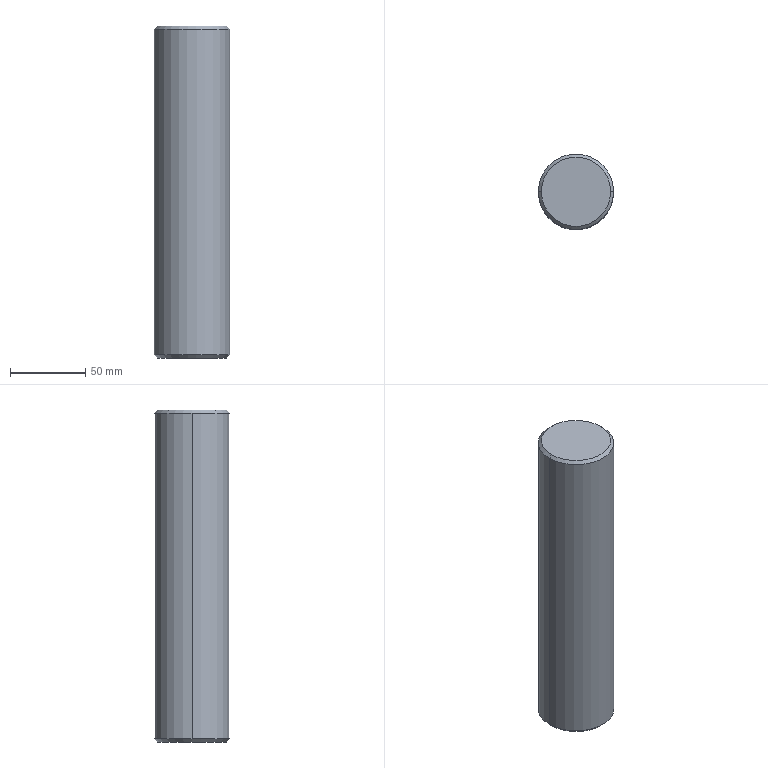Part | SolidWorks | features Chamfer 1, Extrusion 1 | 1 solid | 8 faces | box 50 x 50 x 220 mm | volume 431357 mm3 | cone 4 | cylinder 2 | plane 2 | commonest cylinder face diameters 50 x2
STEP:
#1=CARTESIAN_POINT('',(23.,0.,220.));
#2=VERTEX_POINT('',#1);
#3=CARTESIAN_POINT('',(-23.,0.,220.));
#4=VERTEX_POINT('',#3);
#5=CARTESIAN_POINT('',(0.,0.,220.));
#6=DIRECTION('',(0.,0.,1.));
#7=DIRECTION('',(1.,0.,0.));
#8=AXIS2_PLACEMENT_3D('',#5,#6,#7);
#9=CIRCLE('',#8,23.);
#10=EDGE_CURVE('',#2,#4,#9,.T.);
#11=ORIENTED_EDGE('',*,*,#10,.F.);
#12=CARTESIAN_POINT('',(25.,0.,218.));
#13=VERTEX_POINT('',#12);
#14=CARTESIAN_POINT('',(23.,0.,220.));
#15=DIRECTION('',(0.7071,0.,-0.7071));
#16=VECTOR('',#15,1000.);
#17=LINE('',#14,#16);
#18=EDGE_CURVE('',#2,#13,#17,.T.);
#19=ORIENTED_EDGE('',*,*,#18,.T.);
#20=CARTESIAN_POINT('',(-25.,0.,218.));
#21=VERTEX_POINT('',#20);
#22=CARTESIAN_POINT('',(0.,0.,218.));
#23=DIRECTION('',(0.,0.,-1.));
#24=DIRECTION('',(1.,0.,0.));
#25=AXIS2_PLACEMENT_3D('',#22,#23,#24);
#26=CIRCLE('',#25,25.);
#27=EDGE_CURVE('',#21,#13,#26,.T.);
#28=ORIENTED_EDGE('',*,*,#27,.F.);
#29=CARTESIAN_POINT('',(-23.,0.,220.));
#30=DIRECTION('',(-0.7071,0.,-0.7071));
#31=VECTOR('',#30,1000.);
#32=LINE('',#29,#31);
#33=EDGE_CURVE('',#4,#21,#32,.T.);
#34=ORIENTED_EDGE('',*,*,#33,.F.);
#35=EDGE_LOOP('',(#11,#19,#28,#34));
#36=FACE_OUTER_BOUND('',#35,.T.);
#37=CARTESIAN_POINT('',(0.,0.,220.));
#38=DIRECTION('',(0.,0.,-1.));
#39=DIRECTION('',(-1.,0.,0.));
#40=AXIS2_PLACEMENT_3D('',#37,#38,#39);
#41=CONICAL_SURFACE('',#40,23.,0.7854);
#42=ADVANCED_FACE('',(#36),#41,.T.);
#43=CARTESIAN_POINT('',(-23.,0.,0.));
#44=VERTEX_POINT('',#43);
#45=CARTESIAN_POINT('',(23.,0.,0.));
#46=VERTEX_POINT('',#45);
#47=CARTESIAN_POINT('',(0.,0.,0.));
#48=DIRECTION('',(0.,0.,-1.));
#49=DIRECTION('',(1.,0.,0.));
#50=AXIS2_PLACEMENT_3D('',#47,#48,#49);
#51=CIRCLE('',#50,23.);
#52=EDGE_CURVE('',#44,#46,#51,.T.);
#53=ORIENTED_EDGE('',*,*,#52,.F.);
#54=CARTESIAN_POINT('',(-25.,0.,2.));
#55=VERTEX_POINT('',#54);
#56=CARTESIAN_POINT('',(-25.,0.,2.));
#57=DIRECTION('',(-0.7071,0.,0.7071));
#58=VECTOR('',#57,1000.);
#59=LINE('',#56,#58);
#60=EDGE_CURVE('',#44,#55,#59,.T.);
#61=ORIENTED_EDGE('',*,*,#60,.T.);
#62=CARTESIAN_POINT('',(25.,0.,2.));
#63=VERTEX_POINT('',#62);
#64=CARTESIAN_POINT('',(0.,0.,2.));
#65=DIRECTION('',(0.,0.,1.));
#66=DIRECTION('',(1.,0.,0.));
#67=AXIS2_PLACEMENT_3D('',#64,#65,#66);
#68=CIRCLE('',#67,25.);
#69=EDGE_CURVE('',#63,#55,#68,.T.);
#70=ORIENTED_EDGE('',*,*,#69,.F.);
#71=CARTESIAN_POINT('',(25.,0.,2.));
#72=DIRECTION('',(0.7071,0.,0.7071));
#73=VECTOR('',#72,1000.);
#74=LINE('',#71,#73);
#75=EDGE_CURVE('',#46,#63,#74,.T.);
#76=ORIENTED_EDGE('',*,*,#75,.F.);
#77=EDGE_LOOP('',(#53,#61,#70,#76));
#78=FACE_OUTER_BOUND('',#77,.T.);
#79=CARTESIAN_POINT('',(0.,0.,2.));
#80=DIRECTION('',(0.,0.,1.));
#81=DIRECTION('',(1.,0.,0.));
#82=AXIS2_PLACEMENT_3D('',#79,#80,#81);
#83=CONICAL_SURFACE('',#82,25.,0.7854);
#84=ADVANCED_FACE('',(#78),#83,.T.);
#85=ORIENTED_EDGE('',*,*,#27,.T.);
#86=CARTESIAN_POINT('',(25.,0.,220.));
#87=DIRECTION('',(0.,0.,-1.));
#88=VECTOR('',#87,1000.);
#89=LINE('',#86,#88);
#90=EDGE_CURVE('',#13,#63,#89,.T.);
#91=ORIENTED_EDGE('',*,*,#90,.T.);
#92=ORIENTED_EDGE('',*,*,#69,.T.);
#93=CARTESIAN_POINT('',(-25.,0.,220.));
#94=DIRECTION('',(0.,0.,-1.));
#95=VECTOR('',#94,1000.);
#96=LINE('',#93,#95);
#97=EDGE_CURVE('',#21,#55,#96,.T.);
#98=ORIENTED_EDGE('',*,*,#97,.F.);
#99=EDGE_LOOP('',(#85,#91,#92,#98));
#100=FACE_OUTER_BOUND('',#99,.T.);
#101=CARTESIAN_POINT('',(0.,0.,220.));
#102=DIRECTION('',(0.,0.,-1.));
#103=DIRECTION('',(-1.,0.,0.));
#104=AXIS2_PLACEMENT_3D('',#101,#102,#103);
#105=CYLINDRICAL_SURFACE('',#104,25.);
#106=ADVANCED_FACE('',(#100),#105,.T.);
#107=ORIENTED_EDGE('',*,*,#90,.F.);
#108=CARTESIAN_POINT('',(0.,0.,218.));
#109=DIRECTION('',(0.,0.,-1.));
#110=DIRECTION('',(1.,0.,0.));
#111=AXIS2_PLACEMENT_3D('',#108,#109,#110);
#112=CIRCLE('',#111,25.);
#113=EDGE_CURVE('',#13,#21,#112,.T.);
#114=ORIENTED_EDGE('',*,*,#113,.T.);
#115=ORIENTED_EDGE('',*,*,#97,.T.);
#116=CARTESIAN_POINT('',(0.,0.,2.));
#117=DIRECTION('',(0.,0.,1.));
#118=DIRECTION('',(1.,0.,0.));
#119=AXIS2_PLACEMENT_3D('',#116,#117,#118);
#120=CIRCLE('',#119,25.);
#121=EDGE_CURVE('',#55,#63,#120,.T.);
#122=ORIENTED_EDGE('',*,*,#121,.T.);
#123=EDGE_LOOP('',(#107,#114,#115,#122));
#124=FACE_OUTER_BOUND('',#123,.T.);
#125=CARTESIAN_POINT('',(0.,0.,220.));
#126=DIRECTION('',(0.,0.,-1.));
#127=DIRECTION('',(-1.,0.,0.));
#128=AXIS2_PLACEMENT_3D('',#125,#126,#127);
#129=CYLINDRICAL_SURFACE('',#128,25.);
#130=ADVANCED_FACE('',(#124),#129,.T.);
#131=CARTESIAN_POINT('',(0.,0.,220.));
#132=DIRECTION('',(0.,0.,1.));
#133=DIRECTION('',(1.,0.,0.));
#134=AXIS2_PLACEMENT_3D('',#131,#132,#133);
#135=CIRCLE('',#134,23.);
#136=EDGE_CURVE('',#4,#2,#135,.T.);
#137=ORIENTED_EDGE('',*,*,#136,.T.);
#138=ORIENTED_EDGE('',*,*,#10,.T.);
#139=EDGE_LOOP('',(#137,#138));
#140=FACE_OUTER_BOUND('',#139,.T.);
#141=CARTESIAN_POINT('',(0.,0.,220.));
#142=DIRECTION('',(0.,0.,1.));
#143=DIRECTION('',(1.,0.,0.));
#144=AXIS2_PLACEMENT_3D('',#141,#142,#143);
#145=PLANE('',#144);
#146=ADVANCED_FACE('',(#140),#145,.T.);
#147=CARTESIAN_POINT('',(0.,0.,0.));
#148=DIRECTION('',(0.,0.,-1.));
#149=DIRECTION('',(1.,0.,0.));
#150=AXIS2_PLACEMENT_3D('',#147,#148,#149);
#151=CIRCLE('',#150,23.);
#152=EDGE_CURVE('',#46,#44,#151,.T.);
#153=ORIENTED_EDGE('',*,*,#152,.T.);
#154=ORIENTED_EDGE('',*,*,#52,.T.);
#155=EDGE_LOOP('',(#153,#154));
#156=FACE_OUTER_BOUND('',#155,.T.);
#157=CARTESIAN_POINT('',(0.,0.,0.));
#158=DIRECTION('',(0.,0.,1.));
#159=DIRECTION('',(1.,0.,0.));
#160=AXIS2_PLACEMENT_3D('',#157,#158,#159);
#161=PLANE('',#160);
#162=ADVANCED_FACE('',(#156),#161,.F.);
#163=ORIENTED_EDGE('',*,*,#60,.F.);
#164=ORIENTED_EDGE('',*,*,#152,.F.);
#165=ORIENTED_EDGE('',*,*,#75,.T.);
#166=ORIENTED_EDGE('',*,*,#121,.F.);
#167=EDGE_LOOP('',(#163,#164,#165,#166));
#168=FACE_OUTER_BOUND('',#167,.T.);
#169=CARTESIAN_POINT('',(0.,0.,2.));
#170=DIRECTION('',(0.,0.,1.));
#171=DIRECTION('',(1.,0.,0.));
#172=AXIS2_PLACEMENT_3D('',#169,#170,#171);
#173=CONICAL_SURFACE('',#172,25.,0.7854);
#174=ADVANCED_FACE('',(#168),#173,.T.);
#175=ORIENTED_EDGE('',*,*,#18,.F.);
#176=ORIENTED_EDGE('',*,*,#136,.F.);
#177=ORIENTED_EDGE('',*,*,#33,.T.);
#178=ORIENTED_EDGE('',*,*,#113,.F.);
#179=EDGE_LOOP('',(#175,#176,#177,#178));
#180=FACE_OUTER_BOUND('',#179,.T.);
#181=CARTESIAN_POINT('',(0.,0.,220.));
#182=DIRECTION('',(0.,0.,-1.));
#183=DIRECTION('',(-1.,0.,0.));
#184=AXIS2_PLACEMENT_3D('',#181,#182,#183);
#185=CONICAL_SURFACE('',#184,23.,0.7854);
#186=ADVANCED_FACE('',(#180),#185,.T.);
#187=CLOSED_SHELL('',(#42,#84,#106,#130,#146,#162,#174,#186));
#188=MANIFOLD_SOLID_BREP('',#187);
#189=CARTESIAN_POINT('',(0.,0.,0.));
#190=DIRECTION('',(0.,0.,1.));
#191=DIRECTION('',(1.,0.,0.));
#192=AXIS2_PLACEMENT_3D('',#189,#190,#191);
#193=(LENGTH_UNIT()NAMED_UNIT(*)SI_UNIT(.MILLI.,.METRE.));
#194=UNCERTAINTY_MEASURE_WITH_UNIT(LENGTH_MEASURE(0.00001),#193,'','');
#195=(NAMED_UNIT(*)PLANE_ANGLE_UNIT()SI_UNIT($,.RADIAN.));
#196=(NAMED_UNIT(*)SI_UNIT($,.STERADIAN.)SOLID_ANGLE_UNIT());
#197=(GEOMETRIC_REPRESENTATION_CONTEXT(3)GLOBAL_UNCERTAINTY_ASSIGNED_CONTEXT((#194))GLOBAL_UNIT_ASSIGNED_CONTEXT((#193,#195,#196))REPRESENTATION_CONTEXT('',''));
#198=ADVANCED_BREP_SHAPE_REPRESENTATION('',(#188,#192),#197);